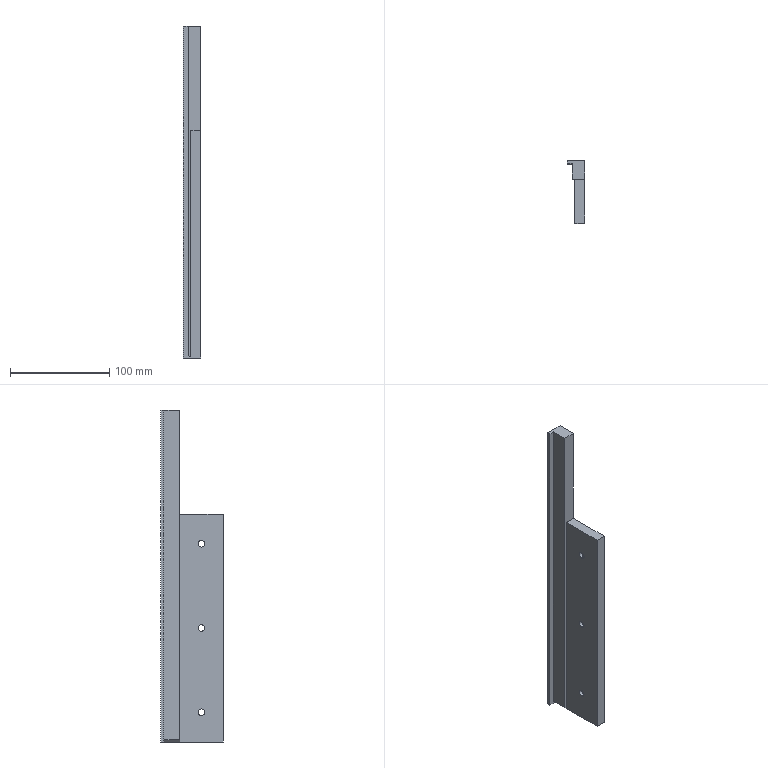Part | STEP file | Side stopper bar | 1 solid | 27 faces | box 17.5 x 63 x 335 mm | volume 183470 mm3 | plane 15 | cylinder 12 | commonest cylinder face diameters 6.6 x6 11 x6